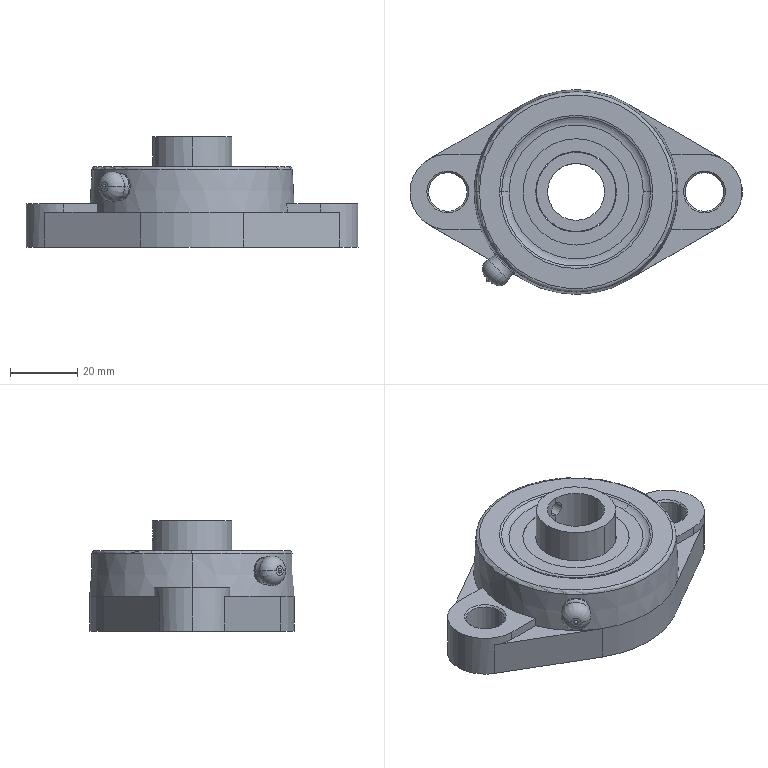Part | SolidWorks | features BaseBody 1 | 1 solid | 105 faces | box 99 x 61 x 32.9 mm | volume 54285 mm3 | cylinder 42 | plane 33 | torus 12 | cone 10 | sphere 8 | commonest cylinder face diameters 6 x6 22.5 x6 31.72 x6 11.5 x4 24.07 x4 4.307 x2